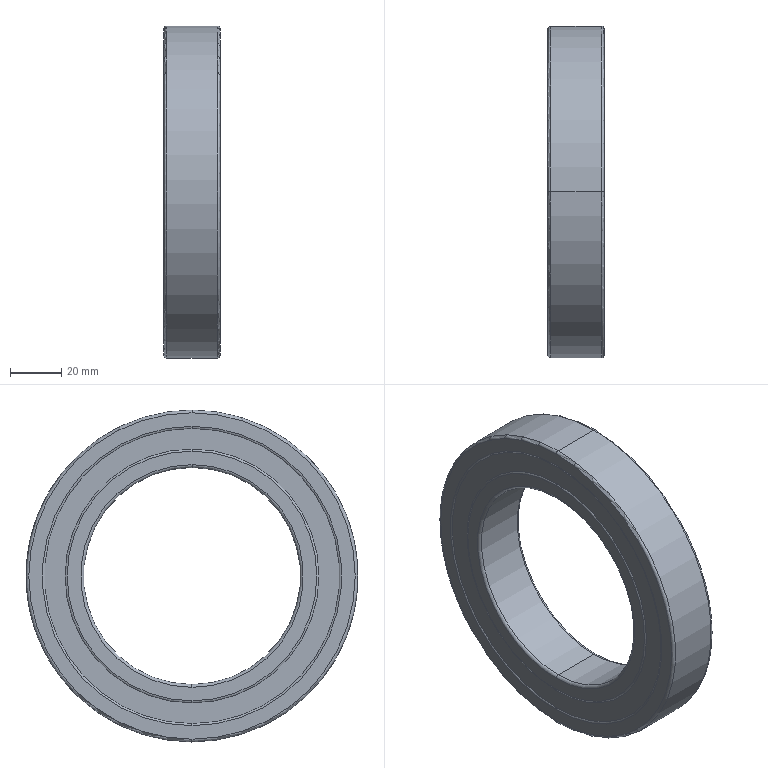Part | SolidWorks | features BaseBody 26 | 26 solids | 286 faces | box 22 x 130 x 130 mm | volume 128128 mm3 | cylinder 106 | sphere 98 | plane 56 | torus 26 | commonest cylinder face diameters 105.25 x47 109.75 x47 100 x4 115 x4 85 x2 130 x2